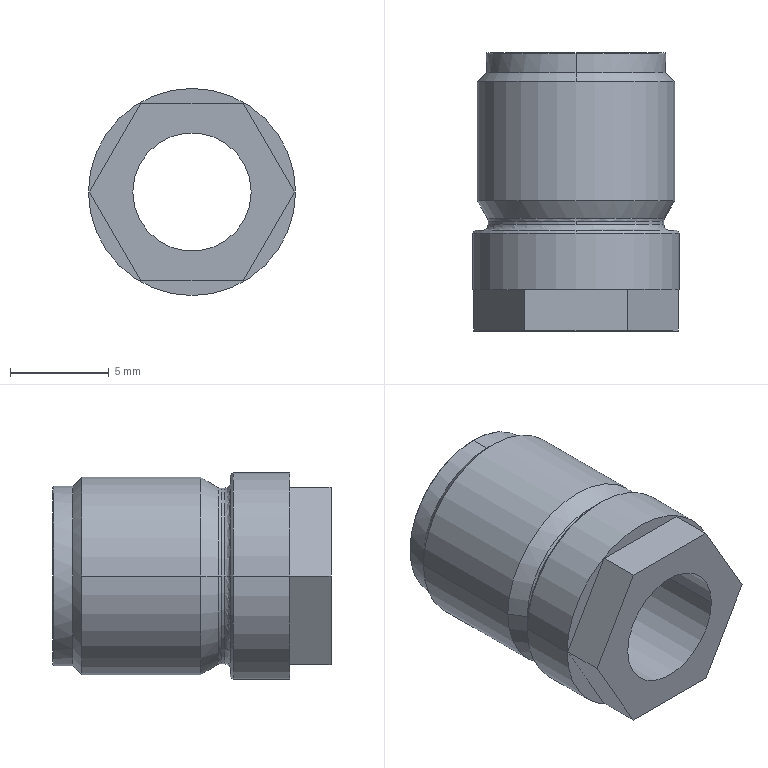Part | STEP file | export_nozzle | 1 solid | 32 faces | box 10.5 x 14.1 x 10.5 mm | volume 682.036 mm3 | cylinder 10 | plane 9 | cone 8 | spline 5 | commonest cylinder face diameters 6 x2 8.9 x2 9.1 x2 10 x2 10.5 x2